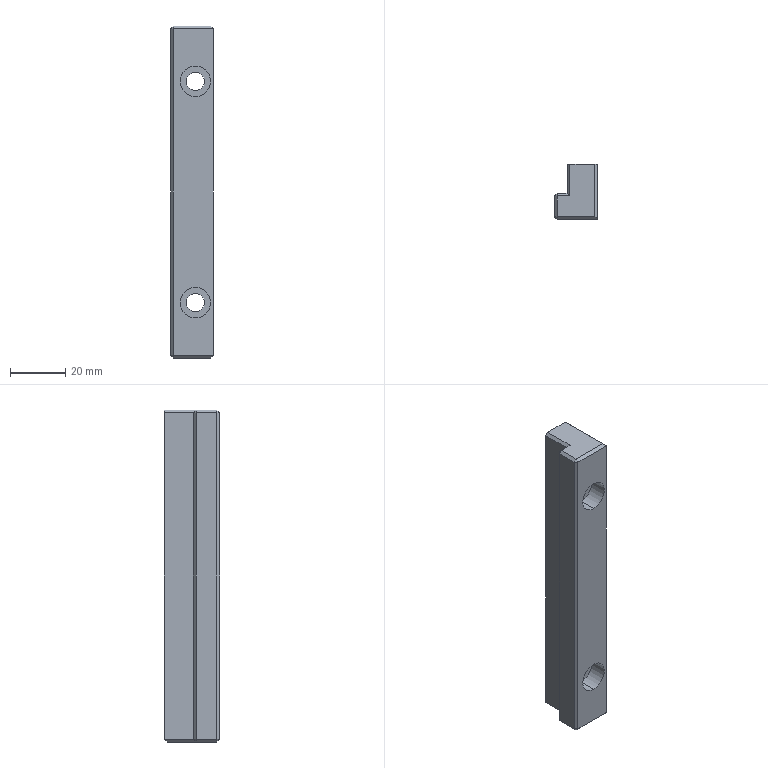Part | STEP file | LM-05-1228 | 1 solid | 35 faces | box 15.5 x 20 x 120 mm | volume 29201 mm3 | plane 27 | cylinder 8 | commonest cylinder face diameters 6.6 x4 11 x4